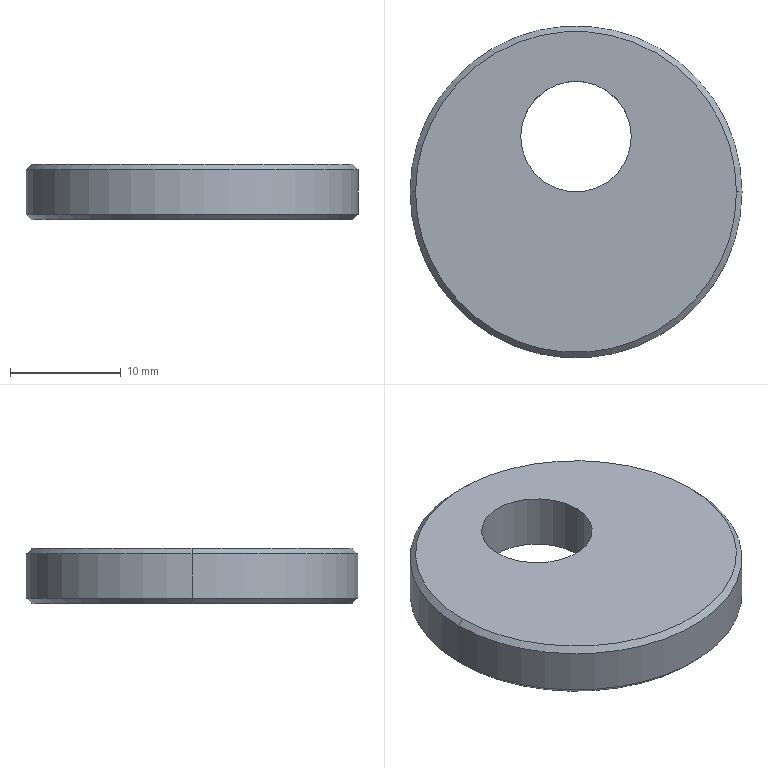Part | SolidWorks | features Chamfer 1, Extrusion 1, ICE 1 | 1 solid | 10 faces | box 30 x 30 x 5 mm | volume 3118 mm3 | cone 4 | cylinder 4 | plane 2 | commonest cylinder face diameters 10 x2 30 x2
STEP:
#1=CARTESIAN_POINT('',(14.5,0.,5.));
#2=VERTEX_POINT('',#1);
#3=CARTESIAN_POINT('',(-14.5,0.,5.));
#4=VERTEX_POINT('',#3);
#5=CARTESIAN_POINT('',(0.,0.,5.));
#6=DIRECTION('',(0.,0.,1.));
#7=DIRECTION('',(1.,0.,0.));
#8=AXIS2_PLACEMENT_3D('',#5,#6,#7);
#9=CIRCLE('',#8,14.5);
#10=EDGE_CURVE('',#2,#4,#9,.T.);
#11=ORIENTED_EDGE('',*,*,#10,.F.);
#12=CARTESIAN_POINT('',(15.,0.,4.5));
#13=VERTEX_POINT('',#12);
#14=CARTESIAN_POINT('',(14.5,0.,5.));
#15=DIRECTION('',(0.7071,0.,-0.7071));
#16=VECTOR('',#15,1000.);
#17=LINE('',#14,#16);
#18=EDGE_CURVE('',#2,#13,#17,.T.);
#19=ORIENTED_EDGE('',*,*,#18,.T.);
#20=CARTESIAN_POINT('',(-15.,0.,4.5));
#21=VERTEX_POINT('',#20);
#22=CARTESIAN_POINT('',(0.,0.,4.5));
#23=DIRECTION('',(0.,0.,-1.));
#24=DIRECTION('',(1.,0.,0.));
#25=AXIS2_PLACEMENT_3D('',#22,#23,#24);
#26=CIRCLE('',#25,15.);
#27=EDGE_CURVE('',#21,#13,#26,.T.);
#28=ORIENTED_EDGE('',*,*,#27,.F.);
#29=CARTESIAN_POINT('',(-14.5,0.,5.));
#30=DIRECTION('',(-0.7071,0.,-0.7071));
#31=VECTOR('',#30,1000.);
#32=LINE('',#29,#31);
#33=EDGE_CURVE('',#4,#21,#32,.T.);
#34=ORIENTED_EDGE('',*,*,#33,.F.);
#35=EDGE_LOOP('',(#11,#19,#28,#34));
#36=FACE_OUTER_BOUND('',#35,.T.);
#37=CARTESIAN_POINT('',(0.,0.,5.));
#38=DIRECTION('',(0.,0.,-1.));
#39=DIRECTION('',(-1.,0.,0.));
#40=AXIS2_PLACEMENT_3D('',#37,#38,#39);
#41=CONICAL_SURFACE('',#40,14.5,0.7854);
#42=ADVANCED_FACE('',(#36),#41,.T.);
#43=CARTESIAN_POINT('',(-14.5,0.,0.));
#44=VERTEX_POINT('',#43);
#45=CARTESIAN_POINT('',(14.5,0.,0.));
#46=VERTEX_POINT('',#45);
#47=CARTESIAN_POINT('',(0.,0.,0.));
#48=DIRECTION('',(0.,0.,-1.));
#49=DIRECTION('',(1.,0.,0.));
#50=AXIS2_PLACEMENT_3D('',#47,#48,#49);
#51=CIRCLE('',#50,14.5);
#52=EDGE_CURVE('',#44,#46,#51,.T.);
#53=ORIENTED_EDGE('',*,*,#52,.F.);
#54=CARTESIAN_POINT('',(-15.,0.,0.5));
#55=VERTEX_POINT('',#54);
#56=CARTESIAN_POINT('',(-15.,0.,0.5));
#57=DIRECTION('',(-0.7071,0.,0.7071));
#58=VECTOR('',#57,1000.);
#59=LINE('',#56,#58);
#60=EDGE_CURVE('',#44,#55,#59,.T.);
#61=ORIENTED_EDGE('',*,*,#60,.T.);
#62=CARTESIAN_POINT('',(15.,0.,0.5));
#63=VERTEX_POINT('',#62);
#64=CARTESIAN_POINT('',(0.,0.,0.5));
#65=DIRECTION('',(0.,0.,1.));
#66=DIRECTION('',(1.,0.,0.));
#67=AXIS2_PLACEMENT_3D('',#64,#65,#66);
#68=CIRCLE('',#67,15.);
#69=EDGE_CURVE('',#63,#55,#68,.T.);
#70=ORIENTED_EDGE('',*,*,#69,.F.);
#71=CARTESIAN_POINT('',(15.,0.,0.5));
#72=DIRECTION('',(0.7071,0.,0.7071));
#73=VECTOR('',#72,1000.);
#74=LINE('',#71,#73);
#75=EDGE_CURVE('',#46,#63,#74,.T.);
#76=ORIENTED_EDGE('',*,*,#75,.F.);
#77=EDGE_LOOP('',(#53,#61,#70,#76));
#78=FACE_OUTER_BOUND('',#77,.T.);
#79=CARTESIAN_POINT('',(0.,0.,0.5));
#80=DIRECTION('',(0.,0.,1.));
#81=DIRECTION('',(1.,0.,0.));
#82=AXIS2_PLACEMENT_3D('',#79,#80,#81);
#83=CONICAL_SURFACE('',#82,15.,0.7854);
#84=ADVANCED_FACE('',(#78),#83,.T.);
#85=CARTESIAN_POINT('',(-5.,5.,0.));
#86=VERTEX_POINT('',#85);
#87=CARTESIAN_POINT('',(5.,5.,0.));
#88=VERTEX_POINT('',#87);
#89=CARTESIAN_POINT('',(0.,5.,0.));
#90=DIRECTION('',(0.,0.,1.));
#91=DIRECTION('',(1.,0.,0.));
#92=AXIS2_PLACEMENT_3D('',#89,#90,#91);
#93=CIRCLE('',#92,5.);
#94=EDGE_CURVE('',#86,#88,#93,.T.);
#95=ORIENTED_EDGE('',*,*,#94,.F.);
#96=CARTESIAN_POINT('',(-5.,5.,5.));
#97=VERTEX_POINT('',#96);
#98=CARTESIAN_POINT('',(-5.,5.,0.));
#99=DIRECTION('',(0.,0.,1.));
#100=VECTOR('',#99,1000.);
#101=LINE('',#98,#100);
#102=EDGE_CURVE('',#86,#97,#101,.T.);
#103=ORIENTED_EDGE('',*,*,#102,.T.);
#104=CARTESIAN_POINT('',(5.,5.,5.));
#105=VERTEX_POINT('',#104);
#106=CARTESIAN_POINT('',(0.,5.,5.));
#107=DIRECTION('',(0.,0.,1.));
#108=DIRECTION('',(1.,0.,0.));
#109=AXIS2_PLACEMENT_3D('',#106,#107,#108);
#110=CIRCLE('',#109,5.);
#111=EDGE_CURVE('',#97,#105,#110,.T.);
#112=ORIENTED_EDGE('',*,*,#111,.T.);
#113=CARTESIAN_POINT('',(5.,5.,0.));
#114=DIRECTION('',(0.,0.,1.));
#115=VECTOR('',#114,1000.);
#116=LINE('',#113,#115);
#117=EDGE_CURVE('',#88,#105,#116,.T.);
#118=ORIENTED_EDGE('',*,*,#117,.F.);
#119=EDGE_LOOP('',(#95,#103,#112,#118));
#120=FACE_OUTER_BOUND('',#119,.T.);
#121=CARTESIAN_POINT('',(0.,5.,0.));
#122=DIRECTION('',(0.,0.,1.));
#123=DIRECTION('',(1.,0.,0.));
#124=AXIS2_PLACEMENT_3D('',#121,#122,#123);
#125=CYLINDRICAL_SURFACE('',#124,5.);
#126=ADVANCED_FACE('',(#120),#125,.F.);
#127=ORIENTED_EDGE('',*,*,#27,.T.);
#128=CARTESIAN_POINT('',(15.,0.,5.));
#129=DIRECTION('',(0.,0.,-1.));
#130=VECTOR('',#129,1000.);
#131=LINE('',#128,#130);
#132=EDGE_CURVE('',#13,#63,#131,.T.);
#133=ORIENTED_EDGE('',*,*,#132,.T.);
#134=ORIENTED_EDGE('',*,*,#69,.T.);
#135=CARTESIAN_POINT('',(-15.,0.,5.));
#136=DIRECTION('',(0.,0.,-1.));
#137=VECTOR('',#136,1000.);
#138=LINE('',#135,#137);
#139=EDGE_CURVE('',#21,#55,#138,.T.);
#140=ORIENTED_EDGE('',*,*,#139,.F.);
#141=EDGE_LOOP('',(#127,#133,#134,#140));
#142=FACE_OUTER_BOUND('',#141,.T.);
#143=CARTESIAN_POINT('',(0.,0.,5.));
#144=DIRECTION('',(0.,0.,-1.));
#145=DIRECTION('',(-1.,0.,0.));
#146=AXIS2_PLACEMENT_3D('',#143,#144,#145);
#147=CYLINDRICAL_SURFACE('',#146,15.);
#148=ADVANCED_FACE('',(#142),#147,.T.);
#149=ORIENTED_EDGE('',*,*,#132,.F.);
#150=CARTESIAN_POINT('',(0.,0.,4.5));
#151=DIRECTION('',(0.,0.,-1.));
#152=DIRECTION('',(1.,0.,0.));
#153=AXIS2_PLACEMENT_3D('',#150,#151,#152);
#154=CIRCLE('',#153,15.);
#155=EDGE_CURVE('',#13,#21,#154,.T.);
#156=ORIENTED_EDGE('',*,*,#155,.T.);
#157=ORIENTED_EDGE('',*,*,#139,.T.);
#158=CARTESIAN_POINT('',(0.,0.,0.5));
#159=DIRECTION('',(0.,0.,1.));
#160=DIRECTION('',(1.,0.,0.));
#161=AXIS2_PLACEMENT_3D('',#158,#159,#160);
#162=CIRCLE('',#161,15.);
#163=EDGE_CURVE('',#55,#63,#162,.T.);
#164=ORIENTED_EDGE('',*,*,#163,.T.);
#165=EDGE_LOOP('',(#149,#156,#157,#164));
#166=FACE_OUTER_BOUND('',#165,.T.);
#167=CARTESIAN_POINT('',(0.,0.,5.));
#168=DIRECTION('',(0.,0.,-1.));
#169=DIRECTION('',(-1.,0.,0.));
#170=AXIS2_PLACEMENT_3D('',#167,#168,#169);
#171=CYLINDRICAL_SURFACE('',#170,15.);
#172=ADVANCED_FACE('',(#166),#171,.T.);
#173=CARTESIAN_POINT('',(0.,0.,5.));
#174=DIRECTION('',(0.,0.,1.));
#175=DIRECTION('',(1.,0.,0.));
#176=AXIS2_PLACEMENT_3D('',#173,#174,#175);
#177=CIRCLE('',#176,14.5);
#178=EDGE_CURVE('',#4,#2,#177,.T.);
#179=ORIENTED_EDGE('',*,*,#178,.T.);
#180=ORIENTED_EDGE('',*,*,#10,.T.);
#181=EDGE_LOOP('',(#179,#180));
#182=FACE_OUTER_BOUND('',#181,.T.);
#183=CARTESIAN_POINT('',(0.,5.,5.));
#184=DIRECTION('',(0.,0.,1.));
#185=DIRECTION('',(1.,0.,0.));
#186=AXIS2_PLACEMENT_3D('',#183,#184,#185);
#187=CIRCLE('',#186,5.);
#188=EDGE_CURVE('',#105,#97,#187,.T.);
#189=ORIENTED_EDGE('',*,*,#188,.F.);
#190=ORIENTED_EDGE('',*,*,#111,.F.);
#191=EDGE_LOOP('',(#189,#190));
#192=FACE_BOUND('',#191,.T.);
#193=CARTESIAN_POINT('',(0.,0.,5.));
#194=DIRECTION('',(0.,0.,1.));
#195=DIRECTION('',(1.,0.,0.));
#196=AXIS2_PLACEMENT_3D('',#193,#194,#195);
#197=PLANE('',#196);
#198=ADVANCED_FACE('',(#182,#192),#197,.T.);
#199=CARTESIAN_POINT('',(0.,0.,0.));
#200=DIRECTION('',(0.,0.,-1.));
#201=DIRECTION('',(1.,0.,0.));
#202=AXIS2_PLACEMENT_3D('',#199,#200,#201);
#203=CIRCLE('',#202,14.5);
#204=EDGE_CURVE('',#46,#44,#203,.T.);
#205=ORIENTED_EDGE('',*,*,#204,.T.);
#206=ORIENTED_EDGE('',*,*,#52,.T.);
#207=EDGE_LOOP('',(#205,#206));
#208=FACE_OUTER_BOUND('',#207,.T.);
#209=CARTESIAN_POINT('',(0.,5.,0.));
#210=DIRECTION('',(0.,0.,1.));
#211=DIRECTION('',(1.,0.,0.));
#212=AXIS2_PLACEMENT_3D('',#209,#210,#211);
#213=CIRCLE('',#212,5.);
#214=EDGE_CURVE('',#88,#86,#213,.T.);
#215=ORIENTED_EDGE('',*,*,#214,.T.);
#216=ORIENTED_EDGE('',*,*,#94,.T.);
#217=EDGE_LOOP('',(#215,#216));
#218=FACE_BOUND('',#217,.T.);
#219=CARTESIAN_POINT('',(0.,0.,0.));
#220=DIRECTION('',(0.,0.,1.));
#221=DIRECTION('',(1.,0.,0.));
#222=AXIS2_PLACEMENT_3D('',#219,#220,#221);
#223=PLANE('',#222);
#224=ADVANCED_FACE('',(#208,#218),#223,.F.);
#225=ORIENTED_EDGE('',*,*,#102,.F.);
#226=ORIENTED_EDGE('',*,*,#214,.F.);
#227=ORIENTED_EDGE('',*,*,#117,.T.);
#228=ORIENTED_EDGE('',*,*,#188,.T.);
#229=EDGE_LOOP('',(#225,#226,#227,#228));
#230=FACE_OUTER_BOUND('',#229,.T.);
#231=CARTESIAN_POINT('',(0.,5.,0.));
#232=DIRECTION('',(0.,0.,1.));
#233=DIRECTION('',(1.,0.,0.));
#234=AXIS2_PLACEMENT_3D('',#231,#232,#233);
#235=CYLINDRICAL_SURFACE('',#234,5.);
#236=ADVANCED_FACE('',(#230),#235,.F.);
#237=ORIENTED_EDGE('',*,*,#60,.F.);
#238=ORIENTED_EDGE('',*,*,#204,.F.);
#239=ORIENTED_EDGE('',*,*,#75,.T.);
#240=ORIENTED_EDGE('',*,*,#163,.F.);
#241=EDGE_LOOP('',(#237,#238,#239,#240));
#242=FACE_OUTER_BOUND('',#241,.T.);
#243=CARTESIAN_POINT('',(0.,0.,0.5));
#244=DIRECTION('',(0.,0.,1.));
#245=DIRECTION('',(1.,0.,0.));
#246=AXIS2_PLACEMENT_3D('',#243,#244,#245);
#247=CONICAL_SURFACE('',#246,15.,0.7854);
#248=ADVANCED_FACE('',(#242),#247,.T.);
#249=ORIENTED_EDGE('',*,*,#18,.F.);
#250=ORIENTED_EDGE('',*,*,#178,.F.);
#251=ORIENTED_EDGE('',*,*,#33,.T.);
#252=ORIENTED_EDGE('',*,*,#155,.F.);
#253=EDGE_LOOP('',(#249,#250,#251,#252));
#254=FACE_OUTER_BOUND('',#253,.T.);
#255=CARTESIAN_POINT('',(0.,0.,5.));
#256=DIRECTION('',(0.,0.,-1.));
#257=DIRECTION('',(-1.,0.,0.));
#258=AXIS2_PLACEMENT_3D('',#255,#256,#257);
#259=CONICAL_SURFACE('',#258,14.5,0.7854);
#260=ADVANCED_FACE('',(#254),#259,.T.);
#261=CLOSED_SHELL('',(#42,#84,#126,#148,#172,#198,#224,#236,#248,#260));
#262=MANIFOLD_SOLID_BREP('',#261);
#263=CARTESIAN_POINT('',(0.,0.,0.));
#264=DIRECTION('',(0.,0.,1.));
#265=DIRECTION('',(1.,0.,0.));
#266=AXIS2_PLACEMENT_3D('',#263,#264,#265);
#267=(LENGTH_UNIT()NAMED_UNIT(*)SI_UNIT(.MILLI.,.METRE.));
#268=UNCERTAINTY_MEASURE_WITH_UNIT(LENGTH_MEASURE(0.00001),#267,'','');
#269=(NAMED_UNIT(*)PLANE_ANGLE_UNIT()SI_UNIT($,.RADIAN.));
#270=(NAMED_UNIT(*)SI_UNIT($,.STERADIAN.)SOLID_ANGLE_UNIT());
#271=(GEOMETRIC_REPRESENTATION_CONTEXT(3)GLOBAL_UNCERTAINTY_ASSIGNED_CONTEXT((#268))GLOBAL_UNIT_ASSIGNED_CONTEXT((#267,#269,#270))REPRESENTATION_CONTEXT('',''));
#272=ADVANCED_BREP_SHAPE_REPRESENTATION('',(#262,#266),#271);